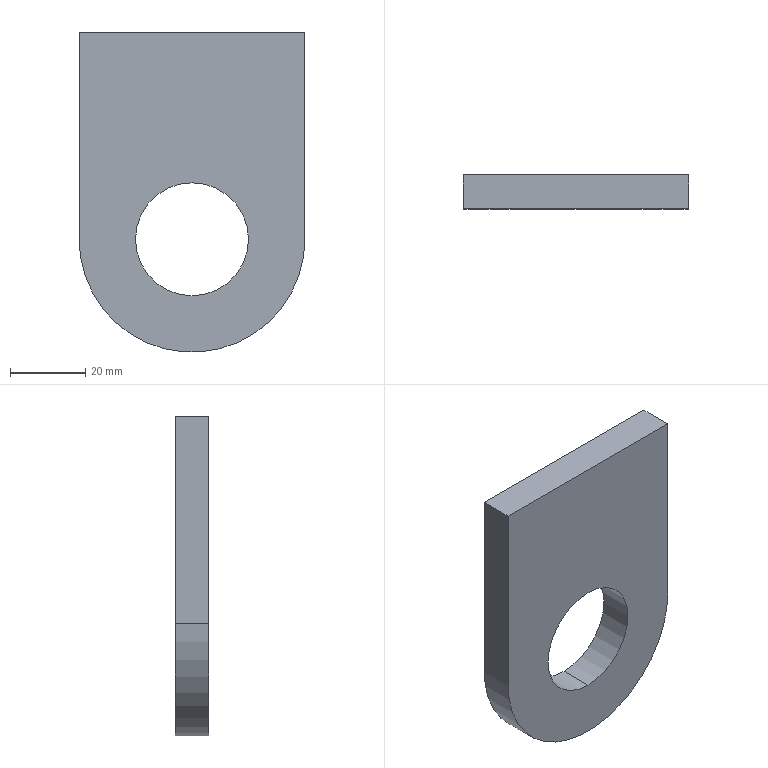Part | SolidWorks | features FlatPattern 1, SMBaseFlange 1, SheetMetal 1 | 1 solid | 8 faces | box 60 x 9 x 85 mm | volume 36062 mm3 | plane 5 | cylinder 3 | commonest cylinder face diameters 30 x2 60 x1
STEP:
#1=CARTESIAN_POINT('',(0.,-9.,-15.));
#2=VERTEX_POINT('',#1);
#3=CARTESIAN_POINT('',(0.,-9.,15.));
#4=VERTEX_POINT('',#3);
#5=CARTESIAN_POINT('',(0.,-9.,0.));
#6=DIRECTION('',(0.,1.,0.));
#7=DIRECTION('',(0.,0.,1.));
#8=AXIS2_PLACEMENT_3D('',#5,#6,#7);
#9=CIRCLE('',#8,15.);
#10=EDGE_CURVE('',#2,#4,#9,.T.);
#11=ORIENTED_EDGE('',*,*,#10,.F.);
#12=CARTESIAN_POINT('',(0.,0.,-15.));
#13=VERTEX_POINT('',#12);
#14=CARTESIAN_POINT('',(0.,-9.,-15.));
#15=DIRECTION('',(0.,1.,0.));
#16=VECTOR('',#15,1000.);
#17=LINE('',#14,#16);
#18=EDGE_CURVE('',#2,#13,#17,.T.);
#19=ORIENTED_EDGE('',*,*,#18,.T.);
#20=CARTESIAN_POINT('',(0.,0.,15.));
#21=VERTEX_POINT('',#20);
#22=CARTESIAN_POINT('',(0.,0.,0.));
#23=DIRECTION('',(0.,1.,0.));
#24=DIRECTION('',(0.,0.,1.));
#25=AXIS2_PLACEMENT_3D('',#22,#23,#24);
#26=CIRCLE('',#25,15.);
#27=EDGE_CURVE('',#13,#21,#26,.T.);
#28=ORIENTED_EDGE('',*,*,#27,.T.);
#29=CARTESIAN_POINT('',(0.,-9.,15.));
#30=DIRECTION('',(0.,1.,0.));
#31=VECTOR('',#30,1000.);
#32=LINE('',#29,#31);
#33=EDGE_CURVE('',#4,#21,#32,.T.);
#34=ORIENTED_EDGE('',*,*,#33,.F.);
#35=EDGE_LOOP('',(#11,#19,#28,#34));
#36=FACE_OUTER_BOUND('',#35,.T.);
#37=CARTESIAN_POINT('',(0.,-9.,0.));
#38=DIRECTION('',(0.,1.,0.));
#39=DIRECTION('',(0.,0.,1.));
#40=AXIS2_PLACEMENT_3D('',#37,#38,#39);
#41=CYLINDRICAL_SURFACE('',#40,15.);
#42=ADVANCED_FACE('',(#36),#41,.F.);
#43=CARTESIAN_POINT('',(30.,0.,0.));
#44=VERTEX_POINT('',#43);
#45=CARTESIAN_POINT('',(-30.,0.,0.));
#46=VERTEX_POINT('',#45);
#47=CARTESIAN_POINT('',(0.,0.,0.));
#48=DIRECTION('',(0.,1.,0.));
#49=DIRECTION('',(0.,0.,1.));
#50=AXIS2_PLACEMENT_3D('',#47,#48,#49);
#51=CIRCLE('',#50,30.);
#52=EDGE_CURVE('',#44,#46,#51,.T.);
#53=ORIENTED_EDGE('',*,*,#52,.F.);
#54=CARTESIAN_POINT('',(30.,-9.,0.));
#55=VERTEX_POINT('',#54);
#56=CARTESIAN_POINT('',(30.,-9.,0.));
#57=DIRECTION('',(0.,1.,0.));
#58=VECTOR('',#57,1000.);
#59=LINE('',#56,#58);
#60=EDGE_CURVE('',#55,#44,#59,.T.);
#61=ORIENTED_EDGE('',*,*,#60,.F.);
#62=CARTESIAN_POINT('',(-30.,-9.,0.));
#63=VERTEX_POINT('',#62);
#64=CARTESIAN_POINT('',(0.,-9.,0.));
#65=DIRECTION('',(0.,1.,0.));
#66=DIRECTION('',(0.,0.,1.));
#67=AXIS2_PLACEMENT_3D('',#64,#65,#66);
#68=CIRCLE('',#67,30.);
#69=EDGE_CURVE('',#55,#63,#68,.T.);
#70=ORIENTED_EDGE('',*,*,#69,.T.);
#71=CARTESIAN_POINT('',(-30.,-9.,0.));
#72=DIRECTION('',(0.,1.,0.));
#73=VECTOR('',#72,1000.);
#74=LINE('',#71,#73);
#75=EDGE_CURVE('',#63,#46,#74,.T.);
#76=ORIENTED_EDGE('',*,*,#75,.T.);
#77=EDGE_LOOP('',(#53,#61,#70,#76));
#78=FACE_OUTER_BOUND('',#77,.T.);
#79=CARTESIAN_POINT('',(0.,-9.,0.));
#80=DIRECTION('',(0.,1.,0.));
#81=DIRECTION('',(0.,0.,1.));
#82=AXIS2_PLACEMENT_3D('',#79,#80,#81);
#83=CYLINDRICAL_SURFACE('',#82,30.);
#84=ADVANCED_FACE('',(#78),#83,.T.);
#85=CARTESIAN_POINT('',(30.,0.,55.));
#86=VERTEX_POINT('',#85);
#87=CARTESIAN_POINT('',(30.,0.,55.));
#88=DIRECTION('',(0.,0.,-1.));
#89=VECTOR('',#88,1000.);
#90=LINE('',#87,#89);
#91=EDGE_CURVE('',#86,#44,#90,.T.);
#92=ORIENTED_EDGE('',*,*,#91,.F.);
#93=CARTESIAN_POINT('',(30.,-9.,55.));
#94=VERTEX_POINT('',#93);
#95=CARTESIAN_POINT('',(30.,-9.,55.));
#96=DIRECTION('',(0.,1.,0.));
#97=VECTOR('',#96,1000.);
#98=LINE('',#95,#97);
#99=EDGE_CURVE('',#94,#86,#98,.T.);
#100=ORIENTED_EDGE('',*,*,#99,.F.);
#101=CARTESIAN_POINT('',(30.,-9.,55.));
#102=DIRECTION('',(0.,0.,-1.));
#103=VECTOR('',#102,1000.);
#104=LINE('',#101,#103);
#105=EDGE_CURVE('',#94,#55,#104,.T.);
#106=ORIENTED_EDGE('',*,*,#105,.T.);
#107=ORIENTED_EDGE('',*,*,#60,.T.);
#108=EDGE_LOOP('',(#92,#100,#106,#107));
#109=FACE_OUTER_BOUND('',#108,.T.);
#110=CARTESIAN_POINT('',(30.,-9.,55.));
#111=DIRECTION('',(1.,0.,0.));
#112=DIRECTION('',(0.,0.,-1.));
#113=AXIS2_PLACEMENT_3D('',#110,#111,#112);
#114=PLANE('',#113);
#115=ADVANCED_FACE('',(#109),#114,.T.);
#116=CARTESIAN_POINT('',(-30.,0.,55.));
#117=VERTEX_POINT('',#116);
#118=CARTESIAN_POINT('',(-30.,0.,55.));
#119=DIRECTION('',(1.,0.,0.));
#120=VECTOR('',#119,1000.);
#121=LINE('',#118,#120);
#122=EDGE_CURVE('',#117,#86,#121,.T.);
#123=ORIENTED_EDGE('',*,*,#122,.F.);
#124=CARTESIAN_POINT('',(-30.,-9.,55.));
#125=VERTEX_POINT('',#124);
#126=CARTESIAN_POINT('',(-30.,-9.,55.));
#127=DIRECTION('',(0.,1.,0.));
#128=VECTOR('',#127,1000.);
#129=LINE('',#126,#128);
#130=EDGE_CURVE('',#125,#117,#129,.T.);
#131=ORIENTED_EDGE('',*,*,#130,.F.);
#132=CARTESIAN_POINT('',(-30.,-9.,55.));
#133=DIRECTION('',(1.,0.,0.));
#134=VECTOR('',#133,1000.);
#135=LINE('',#132,#134);
#136=EDGE_CURVE('',#125,#94,#135,.T.);
#137=ORIENTED_EDGE('',*,*,#136,.T.);
#138=ORIENTED_EDGE('',*,*,#99,.T.);
#139=EDGE_LOOP('',(#123,#131,#137,#138));
#140=FACE_OUTER_BOUND('',#139,.T.);
#141=CARTESIAN_POINT('',(-30.,-9.,55.));
#142=DIRECTION('',(0.,0.,1.));
#143=DIRECTION('',(1.,0.,0.));
#144=AXIS2_PLACEMENT_3D('',#141,#142,#143);
#145=PLANE('',#144);
#146=ADVANCED_FACE('',(#140),#145,.T.);
#147=CARTESIAN_POINT('',(-30.,0.,0.));
#148=DIRECTION('',(0.,0.,1.));
#149=VECTOR('',#148,1000.);
#150=LINE('',#147,#149);
#151=EDGE_CURVE('',#46,#117,#150,.T.);
#152=ORIENTED_EDGE('',*,*,#151,.F.);
#153=ORIENTED_EDGE('',*,*,#75,.F.);
#154=CARTESIAN_POINT('',(-30.,-9.,0.));
#155=DIRECTION('',(0.,0.,1.));
#156=VECTOR('',#155,1000.);
#157=LINE('',#154,#156);
#158=EDGE_CURVE('',#63,#125,#157,.T.);
#159=ORIENTED_EDGE('',*,*,#158,.T.);
#160=ORIENTED_EDGE('',*,*,#130,.T.);
#161=EDGE_LOOP('',(#152,#153,#159,#160));
#162=FACE_OUTER_BOUND('',#161,.T.);
#163=CARTESIAN_POINT('',(-30.,-9.,0.));
#164=DIRECTION('',(-1.,0.,0.));
#165=DIRECTION('',(0.,0.,1.));
#166=AXIS2_PLACEMENT_3D('',#163,#164,#165);
#167=PLANE('',#166);
#168=ADVANCED_FACE('',(#162),#167,.T.);
#169=CARTESIAN_POINT('',(0.,-9.,0.));
#170=DIRECTION('',(0.,1.,0.));
#171=DIRECTION('',(0.,0.,1.));
#172=AXIS2_PLACEMENT_3D('',#169,#170,#171);
#173=CIRCLE('',#172,15.);
#174=EDGE_CURVE('',#4,#2,#173,.T.);
#175=ORIENTED_EDGE('',*,*,#174,.T.);
#176=ORIENTED_EDGE('',*,*,#10,.T.);
#177=EDGE_LOOP('',(#175,#176));
#178=FACE_BOUND('',#177,.T.);
#179=ORIENTED_EDGE('',*,*,#69,.F.);
#180=ORIENTED_EDGE('',*,*,#105,.F.);
#181=ORIENTED_EDGE('',*,*,#136,.F.);
#182=ORIENTED_EDGE('',*,*,#158,.F.);
#183=EDGE_LOOP('',(#179,#180,#181,#182));
#184=FACE_OUTER_BOUND('',#183,.T.);
#185=CARTESIAN_POINT('',(0.,-9.,0.));
#186=DIRECTION('',(0.,1.,0.));
#187=DIRECTION('',(0.,0.,1.));
#188=AXIS2_PLACEMENT_3D('',#185,#186,#187);
#189=PLANE('',#188);
#190=ADVANCED_FACE('',(#178,#184),#189,.F.);
#191=CARTESIAN_POINT('',(0.,0.,0.));
#192=DIRECTION('',(0.,1.,0.));
#193=DIRECTION('',(0.,0.,1.));
#194=AXIS2_PLACEMENT_3D('',#191,#192,#193);
#195=CIRCLE('',#194,15.);
#196=EDGE_CURVE('',#21,#13,#195,.T.);
#197=ORIENTED_EDGE('',*,*,#196,.F.);
#198=ORIENTED_EDGE('',*,*,#27,.F.);
#199=EDGE_LOOP('',(#197,#198));
#200=FACE_BOUND('',#199,.T.);
#201=ORIENTED_EDGE('',*,*,#52,.T.);
#202=ORIENTED_EDGE('',*,*,#151,.T.);
#203=ORIENTED_EDGE('',*,*,#122,.T.);
#204=ORIENTED_EDGE('',*,*,#91,.T.);
#205=EDGE_LOOP('',(#201,#202,#203,#204));
#206=FACE_OUTER_BOUND('',#205,.T.);
#207=CARTESIAN_POINT('',(0.,0.,0.));
#208=DIRECTION('',(0.,1.,0.));
#209=DIRECTION('',(0.,0.,1.));
#210=AXIS2_PLACEMENT_3D('',#207,#208,#209);
#211=PLANE('',#210);
#212=ADVANCED_FACE('',(#200,#206),#211,.T.);
#213=ORIENTED_EDGE('',*,*,#18,.F.);
#214=ORIENTED_EDGE('',*,*,#174,.F.);
#215=ORIENTED_EDGE('',*,*,#33,.T.);
#216=ORIENTED_EDGE('',*,*,#196,.T.);
#217=EDGE_LOOP('',(#213,#214,#215,#216));
#218=FACE_OUTER_BOUND('',#217,.T.);
#219=CARTESIAN_POINT('',(0.,-9.,0.));
#220=DIRECTION('',(0.,1.,0.));
#221=DIRECTION('',(0.,0.,1.));
#222=AXIS2_PLACEMENT_3D('',#219,#220,#221);
#223=CYLINDRICAL_SURFACE('',#222,15.);
#224=ADVANCED_FACE('',(#218),#223,.F.);
#225=CLOSED_SHELL('',(#42,#84,#115,#146,#168,#190,#212,#224));
#226=MANIFOLD_SOLID_BREP('',#225);
#227=CARTESIAN_POINT('',(0.,0.,0.));
#228=DIRECTION('',(0.,0.,1.));
#229=DIRECTION('',(1.,0.,0.));
#230=AXIS2_PLACEMENT_3D('',#227,#228,#229);
#231=(LENGTH_UNIT()NAMED_UNIT(*)SI_UNIT(.MILLI.,.METRE.));
#232=UNCERTAINTY_MEASURE_WITH_UNIT(LENGTH_MEASURE(0.00001),#231,'','');
#233=(NAMED_UNIT(*)PLANE_ANGLE_UNIT()SI_UNIT($,.RADIAN.));
#234=(NAMED_UNIT(*)SI_UNIT($,.STERADIAN.)SOLID_ANGLE_UNIT());
#235=(GEOMETRIC_REPRESENTATION_CONTEXT(3)GLOBAL_UNCERTAINTY_ASSIGNED_CONTEXT((#232))GLOBAL_UNIT_ASSIGNED_CONTEXT((#231,#233,#234))REPRESENTATION_CONTEXT('',''));
#236=ADVANCED_BREP_SHAPE_REPRESENTATION('',(#226,#230),#235);